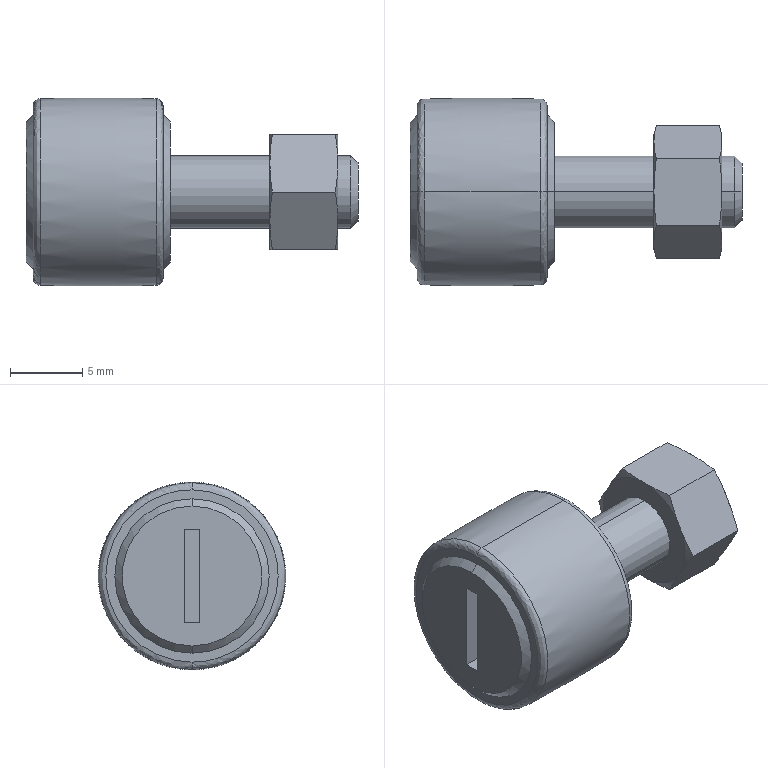Part | STEP file | CFU5-13 | 1 solid | 46 faces | box 23 x 13 x 13 mm | volume 1674 mm3 | plane 18 | cone 18 | spline 4 | cylinder 4 | torus 2 | commonest cylinder face diameters 5 x4
STEP:
#1=CARTESIAN_POINT('',(-0.992,0.,-6.468));
#2=VERTEX_POINT('',#1);
#3=CARTESIAN_POINT('',(-0.992,0.,6.468));
#4=VERTEX_POINT('',#3);
#5=CARTESIAN_POINT('',(-0.992,0.,0.));
#6=DIRECTION('',(-1.,0.,0.));
#7=DIRECTION('',(0.,0.,1.));
#8=AXIS2_PLACEMENT_3D('',#5,#6,#7);
#9=CIRCLE('',#8,6.468);
#10=EDGE_CURVE('',#2,#4,#9,.T.);
#11=ORIENTED_EDGE('',*,*,#10,.F.);
#12=CARTESIAN_POINT('',(-0.5,0.,-5.968));
#13=VERTEX_POINT('',#12);
#14=CARTESIAN_POINT('',(-1.,0.,-5.968));
#15=DIRECTION('',(0.,-1.,0.));
#16=DIRECTION('',(0.,0.,-1.));
#17=AXIS2_PLACEMENT_3D('',#14,#15,#16);
#18=CIRCLE('',#17,0.5);
#19=EDGE_CURVE('',#2,#13,#18,.T.);
#20=ORIENTED_EDGE('',*,*,#19,.T.);
#21=CARTESIAN_POINT('',(-0.5,0.,5.968));
#22=VERTEX_POINT('',#21);
#23=CARTESIAN_POINT('',(-0.5,0.,-5.968));
#24=CARTESIAN_POINT('',(-0.5,-11.936,-5.968));
#25=CARTESIAN_POINT('',(-0.5,-11.936,5.968));
#26=CARTESIAN_POINT('',(-0.5,0.,5.968));
#27=(BOUNDED_CURVE()B_SPLINE_CURVE(3,(#23,#24,#25,#26),.UNSPECIFIED.,.F.,.F.)B_SPLINE_CURVE_WITH_KNOTS((4,4),(0.,1.),.UNSPECIFIED.)CURVE()GEOMETRIC_REPRESENTATION_ITEM()RATIONAL_B_SPLINE_CURVE((1.,0.3333,0.3333,1.))REPRESENTATION_ITEM(''));
#28=EDGE_CURVE('',#13,#22,#27,.T.);
#29=ORIENTED_EDGE('',*,*,#28,.T.);
#30=CARTESIAN_POINT('',(-1.,0.,5.968));
#31=DIRECTION('',(0.,1.,0.));
#32=DIRECTION('',(0.,0.,1.));
#33=AXIS2_PLACEMENT_3D('',#30,#31,#32);
#34=CIRCLE('',#33,0.5);
#35=EDGE_CURVE('',#4,#22,#34,.T.);
#36=ORIENTED_EDGE('',*,*,#35,.F.);
#37=EDGE_LOOP('',(#11,#20,#29,#36));
#38=FACE_OUTER_BOUND('',#37,.T.);
#39=CARTESIAN_POINT('',(-0.992,0.,-6.468));
#40=CARTESIAN_POINT('',(-0.992,-12.936,-6.468));
#41=CARTESIAN_POINT('',(-0.992,-12.936,6.468));
#42=CARTESIAN_POINT('',(-0.992,0.,6.468));
#43=CARTESIAN_POINT('',(-0.7028,0.,-6.463));
#44=CARTESIAN_POINT('',(-0.7028,-12.926,-6.463));
#45=CARTESIAN_POINT('',(-0.7028,-12.926,6.463));
#46=CARTESIAN_POINT('',(-0.7028,0.,6.463));
#47=CARTESIAN_POINT('',(-0.5,0.,-6.257));
#48=CARTESIAN_POINT('',(-0.5,-12.514,-6.257));
#49=CARTESIAN_POINT('',(-0.5,-12.514,6.257));
#50=CARTESIAN_POINT('',(-0.5,0.,6.257));
#51=CARTESIAN_POINT('',(-0.5,0.,-5.968));
#52=CARTESIAN_POINT('',(-0.5,-11.936,-5.968));
#53=CARTESIAN_POINT('',(-0.5,-11.936,5.968));
#54=CARTESIAN_POINT('',(-0.5,0.,5.968));
#55=(BOUNDED_SURFACE()B_SPLINE_SURFACE(3,3,((#39,#40,#41,#42),(#43,#44,#45,#46),(#47,#48,#49,#50),(#51,#52,#53,#54)),.UNSPECIFIED.,.F.,.F.,.F.)B_SPLINE_SURFACE_WITH_KNOTS((4,4),(4,4),(0.,1.),(0.,1.),.UNSPECIFIED.)GEOMETRIC_REPRESENTATION_ITEM()RATIONAL_B_SPLINE_SURFACE(((1.,0.3333,0.3333,1.),(0.8085,0.2695,0.2695,0.8085),(0.8085,0.2695,0.2695,0.8085),(1.,0.3333,0.3333,1.)))REPRESENTATION_ITEM('')SURFACE());
#56=ADVANCED_FACE('',(#38),#55,.T.);
#57=CARTESIAN_POINT('',(-9.5,-5.968,0.));
#58=VERTEX_POINT('',#57);
#59=CARTESIAN_POINT('',(-9.5,0.,-5.968));
#60=VERTEX_POINT('',#59);
#61=CARTESIAN_POINT('',(-9.5,-5.968,0.));
#62=CARTESIAN_POINT('',(-9.5,-5.968,-3.496));
#63=CARTESIAN_POINT('',(-9.5,-3.496,-5.968));
#64=CARTESIAN_POINT('',(-9.5,0.,-5.968));
#65=(BOUNDED_CURVE()B_SPLINE_CURVE(3,(#61,#62,#63,#64),.UNSPECIFIED.,.F.,.F.)B_SPLINE_CURVE_WITH_KNOTS((4,4),(0.,1.),.UNSPECIFIED.)CURVE()GEOMETRIC_REPRESENTATION_ITEM()RATIONAL_B_SPLINE_CURVE((1.,0.8047,0.8047,1.))REPRESENTATION_ITEM(''));
#66=EDGE_CURVE('',#58,#60,#65,.T.);
#67=ORIENTED_EDGE('',*,*,#66,.T.);
#68=CARTESIAN_POINT('',(-9.008,0.,-6.468));
#69=VERTEX_POINT('',#68);
#70=CARTESIAN_POINT('',(-9.,0.,-5.968));
#71=DIRECTION('',(0.,-1.,0.));
#72=DIRECTION('',(0.,0.,-1.));
#73=AXIS2_PLACEMENT_3D('',#70,#71,#72);
#74=CIRCLE('',#73,0.5);
#75=EDGE_CURVE('',#60,#69,#74,.T.);
#76=ORIENTED_EDGE('',*,*,#75,.T.);
#77=CARTESIAN_POINT('',(-9.008,0.,6.468));
#78=VERTEX_POINT('',#77);
#79=CARTESIAN_POINT('',(-9.008,0.,0.));
#80=DIRECTION('',(1.,0.,0.));
#81=DIRECTION('',(0.,0.,-1.));
#82=AXIS2_PLACEMENT_3D('',#79,#80,#81);
#83=CIRCLE('',#82,6.468);
#84=EDGE_CURVE('',#78,#69,#83,.T.);
#85=ORIENTED_EDGE('',*,*,#84,.F.);
#86=CARTESIAN_POINT('',(-9.5,0.,5.968));
#87=VERTEX_POINT('',#86);
#88=CARTESIAN_POINT('',(-9.,0.,5.968));
#89=DIRECTION('',(0.,1.,0.));
#90=DIRECTION('',(0.,0.,1.));
#91=AXIS2_PLACEMENT_3D('',#88,#89,#90);
#92=CIRCLE('',#91,0.5);
#93=EDGE_CURVE('',#87,#78,#92,.T.);
#94=ORIENTED_EDGE('',*,*,#93,.F.);
#95=CARTESIAN_POINT('',(-9.5,0.,5.968));
#96=CARTESIAN_POINT('',(-9.5,-3.496,5.968));
#97=CARTESIAN_POINT('',(-9.5,-5.968,3.496));
#98=CARTESIAN_POINT('',(-9.5,-5.968,0.));
#99=(BOUNDED_CURVE()B_SPLINE_CURVE(3,(#95,#96,#97,#98),.UNSPECIFIED.,.F.,.F.)B_SPLINE_CURVE_WITH_KNOTS((4,4),(0.,1.),.UNSPECIFIED.)CURVE()GEOMETRIC_REPRESENTATION_ITEM()RATIONAL_B_SPLINE_CURVE((1.,0.8047,0.8047,1.))REPRESENTATION_ITEM(''));
#100=EDGE_CURVE('',#87,#58,#99,.T.);
#101=ORIENTED_EDGE('',*,*,#100,.T.);
#102=EDGE_LOOP('',(#67,#76,#85,#94,#101));
#103=FACE_OUTER_BOUND('',#102,.T.);
#104=CARTESIAN_POINT('',(-9.5,0.,-5.968));
#105=CARTESIAN_POINT('',(-9.5,-11.936,-5.968));
#106=CARTESIAN_POINT('',(-9.5,-11.936,5.968));
#107=CARTESIAN_POINT('',(-9.5,0.,5.968));
#108=CARTESIAN_POINT('',(-9.5,0.,-6.257));
#109=CARTESIAN_POINT('',(-9.5,-12.514,-6.257));
#110=CARTESIAN_POINT('',(-9.5,-12.514,6.257));
#111=CARTESIAN_POINT('',(-9.5,0.,6.257));
#112=CARTESIAN_POINT('',(-9.297,0.,-6.463));
#113=CARTESIAN_POINT('',(-9.297,-12.926,-6.463));
#114=CARTESIAN_POINT('',(-9.297,-12.926,6.463));
#115=CARTESIAN_POINT('',(-9.297,0.,6.463));
#116=CARTESIAN_POINT('',(-9.008,0.,-6.468));
#117=CARTESIAN_POINT('',(-9.008,-12.936,-6.468));
#118=CARTESIAN_POINT('',(-9.008,-12.936,6.468));
#119=CARTESIAN_POINT('',(-9.008,0.,6.468));
#120=(BOUNDED_SURFACE()B_SPLINE_SURFACE(3,3,((#104,#105,#106,#107),(#108,#109,#110,#111),(#112,#113,#114,#115),(#116,#117,#118,#119)),.UNSPECIFIED.,.F.,.F.,.F.)B_SPLINE_SURFACE_WITH_KNOTS((4,4),(4,4),(0.,1.),(0.,1.),.UNSPECIFIED.)GEOMETRIC_REPRESENTATION_ITEM()RATIONAL_B_SPLINE_SURFACE(((1.,0.3333,0.3333,1.),(0.8085,0.2695,0.2695,0.8085),(0.8085,0.2695,0.2695,0.8085),(1.,0.3333,0.3333,1.)))REPRESENTATION_ITEM('')SURFACE());
#121=ADVANCED_FACE('',(#103),#120,.T.);
#122=CARTESIAN_POINT('',(-0.992,0.,0.));
#123=DIRECTION('',(-1.,0.,0.));
#124=DIRECTION('',(0.,0.,1.));
#125=AXIS2_PLACEMENT_3D('',#122,#123,#124);
#126=CIRCLE('',#125,6.468);
#127=EDGE_CURVE('',#4,#2,#126,.T.);
#128=ORIENTED_EDGE('',*,*,#127,.T.);
#129=CARTESIAN_POINT('',(-5.,0.,243.5));
#130=DIRECTION('',(0.,1.,0.));
#131=DIRECTION('',(0.,0.,1.));
#132=AXIS2_PLACEMENT_3D('',#129,#130,#131);
#133=CIRCLE('',#132,250.);
#134=EDGE_CURVE('',#2,#69,#133,.T.);
#135=ORIENTED_EDGE('',*,*,#134,.T.);
#136=CARTESIAN_POINT('',(-9.008,0.,0.));
#137=DIRECTION('',(1.,0.,0.));
#138=DIRECTION('',(0.,0.,-1.));
#139=AXIS2_PLACEMENT_3D('',#136,#137,#138);
#140=CIRCLE('',#139,6.468);
#141=EDGE_CURVE('',#69,#78,#140,.T.);
#142=ORIENTED_EDGE('',*,*,#141,.T.);
#143=CARTESIAN_POINT('',(-5.,0.,-243.5));
#144=DIRECTION('',(0.,-1.,0.));
#145=DIRECTION('',(0.,0.,-1.));
#146=AXIS2_PLACEMENT_3D('',#143,#144,#145);
#147=CIRCLE('',#146,250.);
#148=EDGE_CURVE('',#4,#78,#147,.T.);
#149=ORIENTED_EDGE('',*,*,#148,.F.);
#150=EDGE_LOOP('',(#128,#135,#142,#149));
#151=FACE_OUTER_BOUND('',#150,.T.);
#152=CARTESIAN_POINT('',(-5.,0.,0.));
#153=DIRECTION('',(-1.,0.,0.));
#154=DIRECTION('',(0.,0.,1.));
#155=AXIS2_PLACEMENT_3D('',#152,#153,#154);
#156=TOROIDAL_SURFACE('',#155,-243.5,250.);
#157=ADVANCED_FACE('',(#151),#156,.T.);
#158=CARTESIAN_POINT('',(0.,0.,4.85));
#159=VERTEX_POINT('',#158);
#160=CARTESIAN_POINT('',(0.,0.,-4.85));
#161=VERTEX_POINT('',#160);
#162=CARTESIAN_POINT('',(0.,0.,0.));
#163=DIRECTION('',(-1.,0.,0.));
#164=DIRECTION('',(0.,0.,1.));
#165=AXIS2_PLACEMENT_3D('',#162,#163,#164);
#166=CIRCLE('',#165,4.85);
#167=EDGE_CURVE('',#159,#161,#166,.T.);
#168=ORIENTED_EDGE('',*,*,#167,.T.);
#169=CARTESIAN_POINT('',(-0.5,0.,-5.35));
#170=VERTEX_POINT('',#169);
#171=CARTESIAN_POINT('',(-0.5,0.,-5.35));
#172=DIRECTION('',(-0.7071,0.,-0.7071));
#173=VECTOR('',#172,1000.);
#174=LINE('',#171,#173);
#175=EDGE_CURVE('',#161,#170,#174,.T.);
#176=ORIENTED_EDGE('',*,*,#175,.T.);
#177=CARTESIAN_POINT('',(-0.5,0.,5.35));
#178=VERTEX_POINT('',#177);
#179=CARTESIAN_POINT('',(-0.5,0.,0.));
#180=DIRECTION('',(-1.,0.,0.));
#181=DIRECTION('',(0.,0.,1.));
#182=AXIS2_PLACEMENT_3D('',#179,#180,#181);
#183=CIRCLE('',#182,5.35);
#184=EDGE_CURVE('',#178,#170,#183,.T.);
#185=ORIENTED_EDGE('',*,*,#184,.F.);
#186=CARTESIAN_POINT('',(-0.5,0.,5.35));
#187=DIRECTION('',(-0.7071,0.,0.7071));
#188=VECTOR('',#187,1000.);
#189=LINE('',#186,#188);
#190=EDGE_CURVE('',#159,#178,#189,.T.);
#191=ORIENTED_EDGE('',*,*,#190,.F.);
#192=EDGE_LOOP('',(#168,#176,#185,#191));
#193=FACE_OUTER_BOUND('',#192,.T.);
#194=CARTESIAN_POINT('',(-0.5,0.,0.));
#195=DIRECTION('',(-1.,0.,0.));
#196=DIRECTION('',(0.,0.,1.));
#197=AXIS2_PLACEMENT_3D('',#194,#195,#196);
#198=CONICAL_SURFACE('',#197,5.35,0.7854);
#199=ADVANCED_FACE('',(#193),#198,.T.);
#200=CARTESIAN_POINT('',(-10.,0.,-4.85));
#201=VERTEX_POINT('',#200);
#202=CARTESIAN_POINT('',(-10.,0.,4.85));
#203=VERTEX_POINT('',#202);
#204=CARTESIAN_POINT('',(-10.,0.,0.));
#205=DIRECTION('',(1.,0.,0.));
#206=DIRECTION('',(0.,0.,-1.));
#207=AXIS2_PLACEMENT_3D('',#204,#205,#206);
#208=CIRCLE('',#207,4.85);
#209=EDGE_CURVE('',#201,#203,#208,.T.);
#210=ORIENTED_EDGE('',*,*,#209,.T.);
#211=CARTESIAN_POINT('',(-9.5,0.,5.35));
#212=VERTEX_POINT('',#211);
#213=CARTESIAN_POINT('',(-9.5,0.,5.35));
#214=DIRECTION('',(0.7071,0.,0.7071));
#215=VECTOR('',#214,1000.);
#216=LINE('',#213,#215);
#217=EDGE_CURVE('',#203,#212,#216,.T.);
#218=ORIENTED_EDGE('',*,*,#217,.T.);
#219=CARTESIAN_POINT('',(-9.5,0.,-5.35));
#220=VERTEX_POINT('',#219);
#221=CARTESIAN_POINT('',(-9.5,0.,0.));
#222=DIRECTION('',(1.,0.,0.));
#223=DIRECTION('',(0.,0.,-1.));
#224=AXIS2_PLACEMENT_3D('',#221,#222,#223);
#225=CIRCLE('',#224,5.35);
#226=EDGE_CURVE('',#220,#212,#225,.T.);
#227=ORIENTED_EDGE('',*,*,#226,.F.);
#228=CARTESIAN_POINT('',(-9.5,0.,-5.35));
#229=DIRECTION('',(0.7071,0.,-0.7071));
#230=VECTOR('',#229,1000.);
#231=LINE('',#228,#230);
#232=EDGE_CURVE('',#201,#220,#231,.T.);
#233=ORIENTED_EDGE('',*,*,#232,.F.);
#234=EDGE_LOOP('',(#210,#218,#227,#233));
#235=FACE_OUTER_BOUND('',#234,.T.);
#236=CARTESIAN_POINT('',(-9.5,0.,0.));
#237=DIRECTION('',(1.,0.,0.));
#238=DIRECTION('',(0.,0.,-1.));
#239=AXIS2_PLACEMENT_3D('',#236,#237,#238);
#240=CONICAL_SURFACE('',#239,5.35,0.7854);
#241=ADVANCED_FACE('',(#235),#240,.T.);
#242=CARTESIAN_POINT('',(0.,0.,2.5));
#243=VERTEX_POINT('',#242);
#244=CARTESIAN_POINT('',(0.,0.,-2.5));
#245=VERTEX_POINT('',#244);
#246=CARTESIAN_POINT('',(0.,0.,0.));
#247=DIRECTION('',(-1.,0.,0.));
#248=DIRECTION('',(0.,0.,-1.));
#249=AXIS2_PLACEMENT_3D('',#246,#247,#248);
#250=CIRCLE('',#249,2.5);
#251=EDGE_CURVE('',#243,#245,#250,.T.);
#252=ORIENTED_EDGE('',*,*,#251,.F.);
#253=CARTESIAN_POINT('',(6.9,0.,2.5));
#254=VERTEX_POINT('',#253);
#255=CARTESIAN_POINT('',(6.255,0.,2.5));
#256=DIRECTION('',(1.,0.,0.));
#257=VECTOR('',#256,1000.);
#258=LINE('',#255,#257);
#259=EDGE_CURVE('',#243,#254,#258,.T.);
#260=ORIENTED_EDGE('',*,*,#259,.T.);
#261=CARTESIAN_POINT('',(6.9,0.,-2.5));
#262=VERTEX_POINT('',#261);
#263=CARTESIAN_POINT('',(6.9,0.,0.));
#264=DIRECTION('',(-1.,0.,0.));
#265=DIRECTION('',(0.,0.,-1.));
#266=AXIS2_PLACEMENT_3D('',#263,#264,#265);
#267=CIRCLE('',#266,2.5);
#268=EDGE_CURVE('',#254,#262,#267,.T.);
#269=ORIENTED_EDGE('',*,*,#268,.T.);
#270=CARTESIAN_POINT('',(6.255,0.,-2.5));
#271=DIRECTION('',(1.,0.,0.));
#272=VECTOR('',#271,1000.);
#273=LINE('',#270,#272);
#274=EDGE_CURVE('',#245,#262,#273,.T.);
#275=ORIENTED_EDGE('',*,*,#274,.F.);
#276=EDGE_LOOP('',(#252,#260,#269,#275));
#277=FACE_OUTER_BOUND('',#276,.T.);
#278=CARTESIAN_POINT('',(6.255,0.,0.));
#279=DIRECTION('',(1.,0.,0.));
#280=DIRECTION('',(0.,0.,-1.));
#281=AXIS2_PLACEMENT_3D('',#278,#279,#280);
#282=CYLINDRICAL_SURFACE('',#281,2.5);
#283=ADVANCED_FACE('',(#277),#282,.T.);
#284=CARTESIAN_POINT('',(11.6,0.,-2.5));
#285=VERTEX_POINT('',#284);
#286=CARTESIAN_POINT('',(11.6,0.,2.5));
#287=VERTEX_POINT('',#286);
#288=CARTESIAN_POINT('',(11.6,0.,0.));
#289=DIRECTION('',(1.,0.,0.));
#290=DIRECTION('',(0.,0.,-1.));
#291=AXIS2_PLACEMENT_3D('',#288,#289,#290);
#292=CIRCLE('',#291,2.5);
#293=EDGE_CURVE('',#285,#287,#292,.T.);
#294=ORIENTED_EDGE('',*,*,#293,.T.);
#295=CARTESIAN_POINT('',(12.509,0.,2.5));
#296=VERTEX_POINT('',#295);
#297=CARTESIAN_POINT('',(6.255,0.,2.5));
#298=DIRECTION('',(1.,0.,0.));
#299=VECTOR('',#298,1000.);
#300=LINE('',#297,#299);
#301=EDGE_CURVE('',#287,#296,#300,.T.);
#302=ORIENTED_EDGE('',*,*,#301,.T.);
#303=CARTESIAN_POINT('',(12.509,0.,-2.5));
#304=VERTEX_POINT('',#303);
#305=CARTESIAN_POINT('',(12.509,0.,0.));
#306=DIRECTION('',(-1.,0.,0.));
#307=DIRECTION('',(0.,0.,-1.));
#308=AXIS2_PLACEMENT_3D('',#305,#306,#307);
#309=CIRCLE('',#308,2.5);
#310=EDGE_CURVE('',#296,#304,#309,.T.);
#311=ORIENTED_EDGE('',*,*,#310,.T.);
#312=CARTESIAN_POINT('',(6.255,0.,-2.5));
#313=DIRECTION('',(1.,0.,0.));
#314=VECTOR('',#313,1000.);
#315=LINE('',#312,#314);
#316=EDGE_CURVE('',#285,#304,#315,.T.);
#317=ORIENTED_EDGE('',*,*,#316,.F.);
#318=EDGE_LOOP('',(#294,#302,#311,#317));
#319=FACE_OUTER_BOUND('',#318,.T.);
#320=CARTESIAN_POINT('',(6.255,0.,0.));
#321=DIRECTION('',(1.,0.,0.));
#322=DIRECTION('',(0.,0.,-1.));
#323=AXIS2_PLACEMENT_3D('',#320,#321,#322);
#324=CYLINDRICAL_SURFACE('',#323,2.5);
#325=ADVANCED_FACE('',(#319),#324,.T.);
#326=CARTESIAN_POINT('',(13.,0.,2.009));
#327=VERTEX_POINT('',#326);
#328=CARTESIAN_POINT('',(13.,0.,-2.009));
#329=VERTEX_POINT('',#328);
#330=CARTESIAN_POINT('',(13.,0.,0.));
#331=DIRECTION('',(-1.,0.,0.));
#332=DIRECTION('',(0.,0.,1.));
#333=AXIS2_PLACEMENT_3D('',#330,#331,#332);
#334=CIRCLE('',#333,2.009);
#335=EDGE_CURVE('',#327,#329,#334,.T.);
#336=ORIENTED_EDGE('',*,*,#335,.T.);
#337=CARTESIAN_POINT('',(12.51,0.,-2.5));
#338=DIRECTION('',(-0.7071,0.,-0.7071));
#339=VECTOR('',#338,1000.);
#340=LINE('',#337,#339);
#341=EDGE_CURVE('',#329,#304,#340,.T.);
#342=ORIENTED_EDGE('',*,*,#341,.T.);
#343=ORIENTED_EDGE('',*,*,#310,.F.);
#344=CARTESIAN_POINT('',(12.51,0.,2.5));
#345=DIRECTION('',(-0.7071,0.,0.7071));
#346=VECTOR('',#345,1000.);
#347=LINE('',#344,#346);
#348=EDGE_CURVE('',#327,#296,#347,.T.);
#349=ORIENTED_EDGE('',*,*,#348,.F.);
#350=EDGE_LOOP('',(#336,#342,#343,#349));
#351=FACE_OUTER_BOUND('',#350,.T.);
#352=CARTESIAN_POINT('',(12.51,0.,0.));
#353=DIRECTION('',(-1.,0.,0.));
#354=DIRECTION('',(0.,0.,1.));
#355=AXIS2_PLACEMENT_3D('',#352,#353,#354);
#356=CONICAL_SURFACE('',#355,2.5,0.7854);
#357=ADVANCED_FACE('',(#351),#356,.T.);
#358=ORIENTED_EDGE('',*,*,#134,.F.);
#359=ORIENTED_EDGE('',*,*,#10,.T.);
#360=ORIENTED_EDGE('',*,*,#148,.T.);
#361=ORIENTED_EDGE('',*,*,#84,.T.);
#362=EDGE_LOOP('',(#358,#359,#360,#361));
#363=FACE_OUTER_BOUND('',#362,.T.);
#364=CARTESIAN_POINT('',(-5.,0.,0.));
#365=DIRECTION('',(-1.,0.,0.));
#366=DIRECTION('',(0.,0.,1.));
#367=AXIS2_PLACEMENT_3D('',#364,#365,#366);
#368=TOROIDAL_SURFACE('',#367,-243.5,250.);
#369=ADVANCED_FACE('',(#363),#368,.T.);
#370=ORIENTED_EDGE('',*,*,#19,.F.);
#371=ORIENTED_EDGE('',*,*,#127,.F.);
#372=ORIENTED_EDGE('',*,*,#35,.T.);
#373=CARTESIAN_POINT('',(-0.5,5.968,0.));
#374=VERTEX_POINT('',#373);
#375=CARTESIAN_POINT('',(-0.5,0.,5.968));
#376=CARTESIAN_POINT('',(-0.5,3.496,5.968));
#377=CARTESIAN_POINT('',(-0.5,5.968,3.496));
#378=CARTESIAN_POINT('',(-0.5,5.968,0.));
#379=(BOUNDED_CURVE()B_SPLINE_CURVE(3,(#375,#376,#377,#378),.UNSPECIFIED.,.F.,.F.)B_SPLINE_CURVE_WITH_KNOTS((4,4),(0.,1.),.UNSPECIFIED.)CURVE()GEOMETRIC_REPRESENTATION_ITEM()RATIONAL_B_SPLINE_CURVE((1.,0.8047,0.8047,1.))REPRESENTATION_ITEM(''));
#380=EDGE_CURVE('',#22,#374,#379,.T.);
#381=ORIENTED_EDGE('',*,*,#380,.T.);
#382=CARTESIAN_POINT('',(-0.5,5.968,0.));
#383=CARTESIAN_POINT('',(-0.5,5.968,-3.496));
#384=CARTESIAN_POINT('',(-0.5,3.496,-5.968));
#385=CARTESIAN_POINT('',(-0.5,0.,-5.968));
#386=(BOUNDED_CURVE()B_SPLINE_CURVE(3,(#382,#383,#384,#385),.UNSPECIFIED.,.F.,.F.)B_SPLINE_CURVE_WITH_KNOTS((4,4),(0.,1.),.UNSPECIFIED.)CURVE()GEOMETRIC_REPRESENTATION_ITEM()RATIONAL_B_SPLINE_CURVE((1.,0.8047,0.8047,1.))REPRESENTATION_ITEM(''));
#387=EDGE_CURVE('',#374,#13,#386,.T.);
#388=ORIENTED_EDGE('',*,*,#387,.T.);
#389=EDGE_LOOP('',(#370,#371,#372,#381,#388));
#390=FACE_OUTER_BOUND('',#389,.T.);
#391=CARTESIAN_POINT('',(-0.992,0.,6.468));
#392=CARTESIAN_POINT('',(-0.992,12.936,6.468));
#393=CARTESIAN_POINT('',(-0.992,12.936,-6.468));
#394=CARTESIAN_POINT('',(-0.992,0.,-6.468));
#395=CARTESIAN_POINT('',(-0.7028,0.,6.463));
#396=CARTESIAN_POINT('',(-0.7028,12.926,6.463));
#397=CARTESIAN_POINT('',(-0.7028,12.926,-6.463));
#398=CARTESIAN_POINT('',(-0.7028,0.,-6.463));
#399=CARTESIAN_POINT('',(-0.5,0.,6.257));
#400=CARTESIAN_POINT('',(-0.5,12.514,6.257));
#401=CARTESIAN_POINT('',(-0.5,12.514,-6.257));
#402=CARTESIAN_POINT('',(-0.5,0.,-6.257));
#403=CARTESIAN_POINT('',(-0.5,0.,5.968));
#404=CARTESIAN_POINT('',(-0.5,11.936,5.968));
#405=CARTESIAN_POINT('',(-0.5,11.936,-5.968));
#406=CARTESIAN_POINT('',(-0.5,0.,-5.968));
#407=(BOUNDED_SURFACE()B_SPLINE_SURFACE(3,3,((#391,#392,#393,#394),(#395,#396,#397,#398),(#399,#400,#401,#402),(#403,#404,#405,#406)),.UNSPECIFIED.,.F.,.F.,.F.)B_SPLINE_SURFACE_WITH_KNOTS((4,4),(4,4),(0.,1.),(0.,1.),.UNSPECIFIED.)GEOMETRIC_REPRESENTATION_ITEM()RATIONAL_B_SPLINE_SURFACE(((1.,0.3333,0.3333,1.),(0.8085,0.2695,0.2695,0.8085),(0.8085,0.2695,0.2695,0.8085),(1.,0.3333,0.3333,1.)))REPRESENTATION_ITEM('')SURFACE());
#408=ADVANCED_FACE('',(#390),#407,.T.);
#409=ORIENTED_EDGE('',*,*,#75,.F.);
#410=CARTESIAN_POINT('',(-9.5,5.968,0.));
#411=VERTEX_POINT('',#410);
#412=CARTESIAN_POINT('',(-9.5,0.,-5.968));
#413=CARTESIAN_POINT('',(-9.5,3.496,-5.968));
#414=CARTESIAN_POINT('',(-9.5,5.968,-3.496));
#415=CARTESIAN_POINT('',(-9.5,5.968,0.));
#416=(BOUNDED_CURVE()B_SPLINE_CURVE(3,(#412,#413,#414,#415),.UNSPECIFIED.,.F.,.F.)B_SPLINE_CURVE_WITH_KNOTS((4,4),(0.,1.),.UNSPECIFIED.)CURVE()GEOMETRIC_REPRESENTATION_ITEM()RATIONAL_B_SPLINE_CURVE((1.,0.8047,0.8047,1.))REPRESENTATION_ITEM(''));
#417=EDGE_CURVE('',#60,#411,#416,.T.);
#418=ORIENTED_EDGE('',*,*,#417,.T.);
#419=CARTESIAN_POINT('',(-9.5,5.968,0.));
#420=CARTESIAN_POINT('',(-9.5,5.968,3.496));
#421=CARTESIAN_POINT('',(-9.5,3.496,5.968));
#422=CARTESIAN_POINT('',(-9.5,0.,5.968));
#423=(BOUNDED_CURVE()B_SPLINE_CURVE(3,(#419,#420,#421,#422),.UNSPECIFIED.,.F.,.T.)B_SPLINE_CURVE_WITH_KNOTS((4,4),(0.,1.),.UNSPECIFIED.)CURVE()GEOMETRIC_REPRESENTATION_ITEM()RATIONAL_B_SPLINE_CURVE((1.,0.8047,0.8047,1.))REPRESENTATION_ITEM(''));
#424=EDGE_CURVE('',#411,#87,#423,.T.);
#425=ORIENTED_EDGE('',*,*,#424,.T.);
#426=ORIENTED_EDGE('',*,*,#93,.T.);
#427=ORIENTED_EDGE('',*,*,#141,.F.);
#428=EDGE_LOOP('',(#409,#418,#425,#426,#427));
#429=FACE_OUTER_BOUND('',#428,.T.);
#430=CARTESIAN_POINT('',(-9.5,0.,5.968));
#431=CARTESIAN_POINT('',(-9.5,11.936,5.968));
#432=CARTESIAN_POINT('',(-9.5,11.936,-5.968));
#433=CARTESIAN_POINT('',(-9.5,0.,-5.968));
#434=CARTESIAN_POINT('',(-9.5,0.,6.257));
#435=CARTESIAN_POINT('',(-9.5,12.514,6.257));
#436=CARTESIAN_POINT('',(-9.5,12.514,-6.257));
#437=CARTESIAN_POINT('',(-9.5,0.,-6.257));
#438=CARTESIAN_POINT('',(-9.297,0.,6.463));
#439=CARTESIAN_POINT('',(-9.297,12.926,6.463));
#440=CARTESIAN_POINT('',(-9.297,12.926,-6.463));
#441=CARTESIAN_POINT('',(-9.297,0.,-6.463));
#442=CARTESIAN_POINT('',(-9.008,0.,6.468));
#443=CARTESIAN_POINT('',(-9.008,12.936,6.468));
#444=CARTESIAN_POINT('',(-9.008,12.936,-6.468));
#445=CARTESIAN_POINT('',(-9.008,0.,-6.468));
#446=(BOUNDED_SURFACE()B_SPLINE_SURFACE(3,3,((#430,#431,#432,#433),(#434,#435,#436,#437),(#438,#439,#440,#441),(#442,#443,#444,#445)),.UNSPECIFIED.,.F.,.F.,.F.)B_SPLINE_SURFACE_WITH_KNOTS((4,4),(4,4),(0.,1.),(0.,1.),.UNSPECIFIED.)GEOMETRIC_REPRESENTATION_ITEM()RATIONAL_B_SPLINE_SURFACE(((1.,0.3333,0.3333,1.),(0.8085,0.2695,0.2695,0.8085),(0.8085,0.2695,0.2695,0.8085),(1.,0.3333,0.3333,1.)))REPRESENTATION_ITEM('')SURFACE());
#447=ADVANCED_FACE('',(#429),#446,.T.);
#448=ORIENTED_EDGE('',*,*,#184,.T.);
#449=CARTESIAN_POINT('',(-0.5,0.,0.));
#450=DIRECTION('',(-1.,0.,0.));
#451=DIRECTION('',(0.,0.,1.));
#452=AXIS2_PLACEMENT_3D('',#449,#450,#451);
#453=CIRCLE('',#452,5.35);
#454=EDGE_CURVE('',#170,#178,#453,.T.);
#455=ORIENTED_EDGE('',*,*,#454,.T.);
#456=EDGE_LOOP('',(#448,#455));
#457=FACE_BOUND('',#456,.T.);
#458=ORIENTED_EDGE('',*,*,#28,.F.);
#459=ORIENTED_EDGE('',*,*,#387,.F.);
#460=ORIENTED_EDGE('',*,*,#380,.F.);
#461=EDGE_LOOP('',(#458,#459,#460));
#462=FACE_OUTER_BOUND('',#461,.T.);
#463=CARTESIAN_POINT('',(-0.5,5.659,0.));
#464=DIRECTION('',(1.,0.,0.));
#465=DIRECTION('',(0.,0.,-1.));
#466=AXIS2_PLACEMENT_3D('',#463,#464,#465);
#467=PLANE('',#466);
#468=ADVANCED_FACE('',(#457,#462),#467,.T.);
#469=ORIENTED_EDGE('',*,*,#226,.T.);
#470=CARTESIAN_POINT('',(-9.5,0.,0.));
#471=DIRECTION('',(1.,0.,0.));
#472=DIRECTION('',(0.,0.,-1.));
#473=AXIS2_PLACEMENT_3D('',#470,#471,#472);
#474=CIRCLE('',#473,5.35);
#475=EDGE_CURVE('',#212,#220,#474,.T.);
#476=ORIENTED_EDGE('',*,*,#475,.T.);
#477=EDGE_LOOP('',(#469,#476));
#478=FACE_BOUND('',#477,.T.);
#479=ORIENTED_EDGE('',*,*,#424,.F.);
#480=ORIENTED_EDGE('',*,*,#417,.F.);
#481=ORIENTED_EDGE('',*,*,#66,.F.);
#482=ORIENTED_EDGE('',*,*,#100,.F.);
#483=EDGE_LOOP('',(#479,#480,#481,#482));
#484=FACE_OUTER_BOUND('',#483,.T.);
#485=CARTESIAN_POINT('',(-9.5,5.659,0.));
#486=DIRECTION('',(-1.,0.,0.));
#487=DIRECTION('',(0.,0.,1.));
#488=AXIS2_PLACEMENT_3D('',#485,#486,#487);
#489=PLANE('',#488);
#490=ADVANCED_FACE('',(#478,#484),#489,.T.);
#491=ORIENTED_EDGE('',*,*,#175,.F.);
#492=CARTESIAN_POINT('',(0.,0.,0.));
#493=DIRECTION('',(-1.,0.,0.));
#494=DIRECTION('',(0.,0.,1.));
#495=AXIS2_PLACEMENT_3D('',#492,#493,#494);
#496=CIRCLE('',#495,4.85);
#497=EDGE_CURVE('',#161,#159,#496,.T.);
#498=ORIENTED_EDGE('',*,*,#497,.T.);
#499=ORIENTED_EDGE('',*,*,#190,.T.);
#500=ORIENTED_EDGE('',*,*,#454,.F.);
#501=EDGE_LOOP('',(#491,#498,#499,#500));
#502=FACE_OUTER_BOUND('',#501,.T.);
#503=CARTESIAN_POINT('',(-0.5,0.,0.));
#504=DIRECTION('',(-1.,0.,0.));
#505=DIRECTION('',(0.,0.,1.));
#506=AXIS2_PLACEMENT_3D('',#503,#504,#505);
#507=CONICAL_SURFACE('',#506,5.35,0.7854);
#508=ADVANCED_FACE('',(#502),#507,.T.);
#509=ORIENTED_EDGE('',*,*,#217,.F.);
#510=CARTESIAN_POINT('',(-10.,0.,0.));
#511=DIRECTION('',(1.,0.,0.));
#512=DIRECTION('',(0.,0.,-1.));
#513=AXIS2_PLACEMENT_3D('',#510,#511,#512);
#514=CIRCLE('',#513,4.85);
#515=EDGE_CURVE('',#203,#201,#514,.T.);
#516=ORIENTED_EDGE('',*,*,#515,.T.);
#517=ORIENTED_EDGE('',*,*,#232,.T.);
#518=ORIENTED_EDGE('',*,*,#475,.F.);
#519=EDGE_LOOP('',(#509,#516,#517,#518));
#520=FACE_OUTER_BOUND('',#519,.T.);
#521=CARTESIAN_POINT('',(-9.5,0.,0.));
#522=DIRECTION('',(1.,0.,0.));
#523=DIRECTION('',(0.,0.,-1.));
#524=AXIS2_PLACEMENT_3D('',#521,#522,#523);
#525=CONICAL_SURFACE('',#524,5.35,0.7854);
#526=ADVANCED_FACE('',(#520),#525,.T.);
#527=CARTESIAN_POINT('',(0.,0.,0.));
#528=DIRECTION('',(-1.,0.,0.));
#529=DIRECTION('',(0.,0.,-1.));
#530=AXIS2_PLACEMENT_3D('',#527,#528,#529);
#531=CIRCLE('',#530,2.5);
#532=EDGE_CURVE('',#245,#243,#531,.T.);
#533=ORIENTED_EDGE('',*,*,#532,.T.);
#534=ORIENTED_EDGE('',*,*,#251,.T.);
#535=EDGE_LOOP('',(#533,#534));
#536=FACE_BOUND('',#535,.T.);
#537=ORIENTED_EDGE('',*,*,#167,.F.);
#538=ORIENTED_EDGE('',*,*,#497,.F.);
#539=EDGE_LOOP('',(#537,#538));
#540=FACE_OUTER_BOUND('',#539,.T.);
#541=CARTESIAN_POINT('',(0.,3.675,0.));
#542=DIRECTION('',(1.,0.,0.));
#543=DIRECTION('',(0.,0.,-1.));
#544=AXIS2_PLACEMENT_3D('',#541,#542,#543);
#545=PLANE('',#544);
#546=ADVANCED_FACE('',(#536,#540),#545,.T.);
#547=CARTESIAN_POINT('',(-10.,-0.5417,-3.25));
#548=VERTEX_POINT('',#547);
#549=CARTESIAN_POINT('',(-10.,0.5417,-3.25));
#550=VERTEX_POINT('',#549);
#551=CARTESIAN_POINT('',(-10.,0.5417,-3.25));
#552=DIRECTION('',(0.,1.,0.));
#553=VECTOR('',#552,1000.);
#554=LINE('',#551,#553);
#555=EDGE_CURVE('',#548,#550,#554,.T.);
#556=ORIENTED_EDGE('',*,*,#555,.T.);
#557=CARTESIAN_POINT('',(-10.,0.5417,3.25));
#558=VERTEX_POINT('',#557);
#559=CARTESIAN_POINT('',(-10.,0.5417,0.));
#560=DIRECTION('',(0.,0.,1.));
#561=VECTOR('',#560,1000.);
#562=LINE('',#559,#561);
#563=EDGE_CURVE('',#550,#558,#562,.T.);
#564=ORIENTED_EDGE('',*,*,#563,.T.);
#565=CARTESIAN_POINT('',(-10.,-0.5417,3.25));
#566=VERTEX_POINT('',#565);
#567=CARTESIAN_POINT('',(-10.,-0.5417,3.25));
#568=DIRECTION('',(0.,-1.,0.));
#569=VECTOR('',#568,1000.);
#570=LINE('',#567,#569);
#571=EDGE_CURVE('',#558,#566,#570,.T.);
#572=ORIENTED_EDGE('',*,*,#571,.T.);
#573=CARTESIAN_POINT('',(-10.,-0.5417,0.));
#574=DIRECTION('',(0.,0.,-1.));
#575=VECTOR('',#574,1000.);
#576=LINE('',#573,#575);
#577=EDGE_CURVE('',#566,#548,#576,.T.);
#578=ORIENTED_EDGE('',*,*,#577,.T.);
#579=EDGE_LOOP('',(#556,#564,#572,#578));
#580=FACE_BOUND('',#579,.T.);
#581=ORIENTED_EDGE('',*,*,#209,.F.);
#582=ORIENTED_EDGE('',*,*,#515,.F.);
#583=EDGE_LOOP('',(#581,#582));
#584=FACE_OUTER_BOUND('',#583,.T.);
#585=CARTESIAN_POINT('',(-10.,2.425,0.));
#586=DIRECTION('',(-1.,0.,0.));
#587=DIRECTION('',(0.,0.,1.));
#588=AXIS2_PLACEMENT_3D('',#585,#586,#587);
#589=PLANE('',#588);
#590=ADVANCED_FACE('',(#580,#584),#589,.T.);
#591=ORIENTED_EDGE('',*,*,#259,.F.);
#592=ORIENTED_EDGE('',*,*,#532,.F.);
#593=ORIENTED_EDGE('',*,*,#274,.T.);
#594=CARTESIAN_POINT('',(6.9,0.,0.));
#595=DIRECTION('',(-1.,0.,0.));
#596=DIRECTION('',(0.,0.,-1.));
#597=AXIS2_PLACEMENT_3D('',#594,#595,#596);
#598=CIRCLE('',#597,2.5);
#599=EDGE_CURVE('',#262,#254,#598,.T.);
#600=ORIENTED_EDGE('',*,*,#599,.T.);
#601=EDGE_LOOP('',(#591,#592,#593,#600));
#602=FACE_OUTER_BOUND('',#601,.T.);
#603=CARTESIAN_POINT('',(6.255,0.,0.));
#604=DIRECTION('',(1.,0.,0.));
#605=DIRECTION('',(0.,0.,-1.));
#606=AXIS2_PLACEMENT_3D('',#603,#604,#605);
#607=CYLINDRICAL_SURFACE('',#606,2.5);
#608=ADVANCED_FACE('',(#602),#607,.T.);
#609=ORIENTED_EDGE('',*,*,#563,.F.);
#610=CARTESIAN_POINT('',(-8.,0.5417,-3.25));
#611=VERTEX_POINT('',#610);
#612=CARTESIAN_POINT('',(-10.,0.5417,-3.25));
#613=DIRECTION('',(-1.,0.,0.));
#614=VECTOR('',#613,1000.);
#615=LINE('',#612,#614);
#616=EDGE_CURVE('',#611,#550,#615,.T.);
#617=ORIENTED_EDGE('',*,*,#616,.F.);
#618=CARTESIAN_POINT('',(-8.,0.5417,3.25));
#619=VERTEX_POINT('',#618);
#620=CARTESIAN_POINT('',(-8.,0.5417,3.25));
#621=DIRECTION('',(0.,0.,-1.));
#622=VECTOR('',#621,1000.);
#623=LINE('',#620,#622);
#624=EDGE_CURVE('',#619,#611,#623,.T.);
#625=ORIENTED_EDGE('',*,*,#624,.F.);
#626=CARTESIAN_POINT('',(-10.,0.5417,3.25));
#627=DIRECTION('',(1.,0.,0.));
#628=VECTOR('',#627,1000.);
#629=LINE('',#626,#628);
#630=EDGE_CURVE('',#558,#619,#629,.T.);
#631=ORIENTED_EDGE('',*,*,#630,.F.);
#632=EDGE_LOOP('',(#609,#617,#625,#631));
#633=FACE_OUTER_BOUND('',#632,.T.);
#634=CARTESIAN_POINT('',(-10.,0.5417,3.25));
#635=DIRECTION('',(0.,1.,0.));
#636=DIRECTION('',(0.,0.,1.));
#637=AXIS2_PLACEMENT_3D('',#634,#635,#636);
#638=PLANE('',#637);
#639=ADVANCED_FACE('',(#633),#638,.F.);
#640=ORIENTED_EDGE('',*,*,#577,.F.);
#641=CARTESIAN_POINT('',(-8.,-0.5417,3.25));
#642=VERTEX_POINT('',#641);
#643=CARTESIAN_POINT('',(-10.,-0.5417,3.25));
#644=DIRECTION('',(-1.,0.,0.));
#645=VECTOR('',#644,1000.);
#646=LINE('',#643,#645);
#647=EDGE_CURVE('',#642,#566,#646,.T.);
#648=ORIENTED_EDGE('',*,*,#647,.F.);
#649=CARTESIAN_POINT('',(-8.,-0.5417,-3.25));
#650=VERTEX_POINT('',#649);
#651=CARTESIAN_POINT('',(-8.,-0.5417,-3.25));
#652=DIRECTION('',(0.,0.,1.));
#653=VECTOR('',#652,1000.);
#654=LINE('',#651,#653);
#655=EDGE_CURVE('',#650,#642,#654,.T.);
#656=ORIENTED_EDGE('',*,*,#655,.F.);
#657=CARTESIAN_POINT('',(-10.,-0.5417,-3.25));
#658=DIRECTION('',(1.,0.,0.));
#659=VECTOR('',#658,1000.);
#660=LINE('',#657,#659);
#661=EDGE_CURVE('',#548,#650,#660,.T.);
#662=ORIENTED_EDGE('',*,*,#661,.F.);
#663=EDGE_LOOP('',(#640,#648,#656,#662));
#664=FACE_OUTER_BOUND('',#663,.T.);
#665=CARTESIAN_POINT('',(-10.,-0.5417,-3.25));
#666=DIRECTION('',(0.,-1.,0.));
#667=DIRECTION('',(0.,0.,-1.));
#668=AXIS2_PLACEMENT_3D('',#665,#666,#667);
#669=PLANE('',#668);
#670=ADVANCED_FACE('',(#664),#669,.F.);
#671=ORIENTED_EDGE('',*,*,#599,.F.);
#672=ORIENTED_EDGE('',*,*,#268,.F.);
#673=EDGE_LOOP('',(#671,#672));
#674=FACE_BOUND('',#673,.T.);
#675=CARTESIAN_POINT('',(6.9,-3.464,-2.));
#676=VERTEX_POINT('',#675);
#677=CARTESIAN_POINT('',(6.9,-3.464,2.));
#678=VERTEX_POINT('',#677);
#679=CARTESIAN_POINT('',(6.9,0.,0.));
#680=DIRECTION('',(-1.,0.,0.));
#681=DIRECTION('',(0.,0.,-1.));
#682=AXIS2_PLACEMENT_3D('',#679,#680,#681);
#683=CIRCLE('',#682,4.);
#684=EDGE_CURVE('',#676,#678,#683,.T.);
#685=ORIENTED_EDGE('',*,*,#684,.T.);
#686=CARTESIAN_POINT('',(6.9,0.,4.));
#687=VERTEX_POINT('',#686);
#688=CARTESIAN_POINT('',(6.9,0.,0.));
#689=DIRECTION('',(-1.,0.,0.));
#690=DIRECTION('',(0.,0.,-1.));
#691=AXIS2_PLACEMENT_3D('',#688,#689,#690);
#692=CIRCLE('',#691,4.);
#693=EDGE_CURVE('',#678,#687,#692,.T.);
#694=ORIENTED_EDGE('',*,*,#693,.T.);
#695=CARTESIAN_POINT('',(6.9,3.464,2.));
#696=VERTEX_POINT('',#695);
#697=CARTESIAN_POINT('',(6.9,0.,0.));
#698=DIRECTION('',(-1.,0.,0.));
#699=DIRECTION('',(0.,0.,-1.));
#700=AXIS2_PLACEMENT_3D('',#697,#698,#699);
#701=CIRCLE('',#700,4.);
#702=EDGE_CURVE('',#687,#696,#701,.T.);
#703=ORIENTED_EDGE('',*,*,#702,.T.);
#704=CARTESIAN_POINT('',(6.9,3.464,-2.));
#705=VERTEX_POINT('',#704);
#706=CARTESIAN_POINT('',(6.9,0.,0.));
#707=DIRECTION('',(-1.,0.,0.));
#708=DIRECTION('',(0.,0.,-1.));
#709=AXIS2_PLACEMENT_3D('',#706,#707,#708);
#710=CIRCLE('',#709,4.);
#711=EDGE_CURVE('',#696,#705,#710,.T.);
#712=ORIENTED_EDGE('',*,*,#711,.T.);
#713=CARTESIAN_POINT('',(6.9,0.,-4.));
#714=VERTEX_POINT('',#713);
#715=CARTESIAN_POINT('',(6.9,0.,0.));
#716=DIRECTION('',(-1.,0.,0.));
#717=DIRECTION('',(0.,0.,-1.));
#718=AXIS2_PLACEMENT_3D('',#715,#716,#717);
#719=CIRCLE('',#718,4.);
#720=EDGE_CURVE('',#705,#714,#719,.T.);
#721=ORIENTED_EDGE('',*,*,#720,.T.);
#722=CARTESIAN_POINT('',(6.9,0.,0.));
#723=DIRECTION('',(-1.,0.,0.));
#724=DIRECTION('',(0.,0.,-1.));
#725=AXIS2_PLACEMENT_3D('',#722,#723,#724);
#726=CIRCLE('',#725,4.);
#727=EDGE_CURVE('',#714,#676,#726,.T.);
#728=ORIENTED_EDGE('',*,*,#727,.T.);
#729=EDGE_LOOP('',(#685,#694,#703,#712,#721,#728));
#730=FACE_OUTER_BOUND('',#729,.T.);
#731=CARTESIAN_POINT('',(6.9,0.,0.));
#732=DIRECTION('',(-1.,0.,0.));
#733=DIRECTION('',(0.,0.,1.));
#734=AXIS2_PLACEMENT_3D('',#731,#732,#733);
#735=PLANE('',#734);
#736=ADVANCED_FACE('',(#674,#730),#735,.T.);
#737=ORIENTED_EDGE('',*,*,#571,.F.);
#738=ORIENTED_EDGE('',*,*,#630,.T.);
#739=CARTESIAN_POINT('',(-8.,-0.5417,3.25));
#740=DIRECTION('',(0.,1.,0.));
#741=VECTOR('',#740,1000.);
#742=LINE('',#739,#741);
#743=EDGE_CURVE('',#642,#619,#742,.T.);
#744=ORIENTED_EDGE('',*,*,#743,.F.);
#745=ORIENTED_EDGE('',*,*,#647,.T.);
#746=EDGE_LOOP('',(#737,#738,#744,#745));
#747=FACE_OUTER_BOUND('',#746,.T.);
#748=CARTESIAN_POINT('',(-10.,-0.5417,3.25));
#749=DIRECTION('',(0.,0.,1.));
#750=DIRECTION('',(1.,0.,0.));
#751=AXIS2_PLACEMENT_3D('',#748,#749,#750);
#752=PLANE('',#751);
#753=ADVANCED_FACE('',(#747),#752,.F.);
#754=ORIENTED_EDGE('',*,*,#555,.F.);
#755=ORIENTED_EDGE('',*,*,#661,.T.);
#756=CARTESIAN_POINT('',(-8.,0.5417,-3.25));
#757=DIRECTION('',(0.,-1.,0.));
#758=VECTOR('',#757,1000.);
#759=LINE('',#756,#758);
#760=EDGE_CURVE('',#611,#650,#759,.T.);
#761=ORIENTED_EDGE('',*,*,#760,.F.);
#762=ORIENTED_EDGE('',*,*,#616,.T.);
#763=EDGE_LOOP('',(#754,#755,#761,#762));
#764=FACE_OUTER_BOUND('',#763,.T.);
#765=CARTESIAN_POINT('',(-10.,0.5417,-3.25));
#766=DIRECTION('',(0.,0.,-1.));
#767=DIRECTION('',(-1.,0.,0.));
#768=AXIS2_PLACEMENT_3D('',#765,#766,#767);
#769=PLANE('',#768);
#770=ADVANCED_FACE('',(#764),#769,.F.);
#771=ORIENTED_EDGE('',*,*,#743,.T.);
#772=ORIENTED_EDGE('',*,*,#624,.T.);
#773=ORIENTED_EDGE('',*,*,#760,.T.);
#774=ORIENTED_EDGE('',*,*,#655,.T.);
#775=EDGE_LOOP('',(#771,#772,#773,#774));
#776=FACE_OUTER_BOUND('',#775,.T.);
#777=CARTESIAN_POINT('',(-8.,0.,0.));
#778=DIRECTION('',(-1.,0.,0.));
#779=DIRECTION('',(0.,0.,1.));
#780=AXIS2_PLACEMENT_3D('',#777,#778,#779);
#781=PLANE('',#780);
#782=ADVANCED_FACE('',(#776),#781,.T.);
#783=CARTESIAN_POINT('',(7.066,-2.309,4.));
#784=VERTEX_POINT('',#783);
#785=CARTESIAN_POINT('',(6.9,-3.464,2.));
#786=CARTESIAN_POINT('',(6.9,-3.077,2.67));
#787=CARTESIAN_POINT('',(6.963,-2.693,3.336));
#788=CARTESIAN_POINT('',(7.066,-2.309,4.));
#789=B_SPLINE_CURVE_WITH_KNOTS('',3,(#785,#786,#787,#788),.UNSPECIFIED.,.F.,.F.,(4,4),(0.,0.002315),.UNSPECIFIED.);
#790=EDGE_CURVE('',#678,#784,#789,.T.);
#791=ORIENTED_EDGE('',*,*,#790,.T.);
#792=CARTESIAN_POINT('',(7.066,-2.309,4.));
#793=CARTESIAN_POINT('',(6.963,-1.543,4.));
#794=CARTESIAN_POINT('',(6.9,-0.7738,4.));
#795=CARTESIAN_POINT('',(6.9,0.,4.));
#796=B_SPLINE_CURVE_WITH_KNOTS('',3,(#792,#793,#794,#795),.UNSPECIFIED.,.F.,.F.,(4,4),(0.,0.002315),.UNSPECIFIED.);
#797=EDGE_CURVE('',#784,#687,#796,.T.);
#798=ORIENTED_EDGE('',*,*,#797,.T.);
#799=ORIENTED_EDGE('',*,*,#693,.F.);
#800=EDGE_LOOP('',(#791,#798,#799));
#801=FACE_OUTER_BOUND('',#800,.T.);
#802=CARTESIAN_POINT('',(7.067,0.,0.));
#803=DIRECTION('',(1.,0.,0.));
#804=DIRECTION('',(0.,0.,-1.));
#805=AXIS2_PLACEMENT_3D('',#802,#803,#804);
#806=CONICAL_SURFACE('',#805,4.623,1.309);
#807=ADVANCED_FACE('',(#801),#806,.T.);
#808=CARTESIAN_POINT('',(7.066,-4.619,-0.00000002));
#809=VERTEX_POINT('',#808);
#810=CARTESIAN_POINT('',(6.9,-3.464,-2.));
#811=CARTESIAN_POINT('',(6.9,-3.851,-1.33));
#812=CARTESIAN_POINT('',(6.963,-4.236,-0.6637));
#813=CARTESIAN_POINT('',(7.066,-4.619,-0.00000002));
#814=B_SPLINE_CURVE_WITH_KNOTS('',3,(#810,#811,#812,#813),.UNSPECIFIED.,.F.,.F.,(4,4),(0.,0.002315),.UNSPECIFIED.);
#815=EDGE_CURVE('',#676,#809,#814,.T.);
#816=ORIENTED_EDGE('',*,*,#815,.T.);
#817=CARTESIAN_POINT('',(7.066,-4.619,-0.00000002));
#818=CARTESIAN_POINT('',(6.963,-4.236,0.6637));
#819=CARTESIAN_POINT('',(6.9,-3.851,1.33));
#820=CARTESIAN_POINT('',(6.9,-3.464,2.));
#821=B_SPLINE_CURVE_WITH_KNOTS('',3,(#817,#818,#819,#820),.UNSPECIFIED.,.F.,.F.,(4,4),(0.,0.002315),.UNSPECIFIED.);
#822=EDGE_CURVE('',#809,#678,#821,.T.);
#823=ORIENTED_EDGE('',*,*,#822,.T.);
#824=ORIENTED_EDGE('',*,*,#684,.F.);
#825=EDGE_LOOP('',(#816,#823,#824));
#826=FACE_OUTER_BOUND('',#825,.T.);
#827=CARTESIAN_POINT('',(7.067,0.,0.));
#828=DIRECTION('',(1.,0.,0.));
#829=DIRECTION('',(0.,0.,-1.));
#830=AXIS2_PLACEMENT_3D('',#827,#828,#829);
#831=CONICAL_SURFACE('',#830,4.623,1.309);
#832=ADVANCED_FACE('',(#826),#831,.T.);
#833=ORIENTED_EDGE('',*,*,#727,.F.);
#834=CARTESIAN_POINT('',(7.066,-2.309,-4.));
#835=VERTEX_POINT('',#834);
#836=CARTESIAN_POINT('',(6.9,0.,-4.));
#837=CARTESIAN_POINT('',(6.9,-0.7738,-4.));
#838=CARTESIAN_POINT('',(6.963,-1.543,-4.));
#839=CARTESIAN_POINT('',(7.066,-2.309,-4.));
#840=B_SPLINE_CURVE_WITH_KNOTS('',3,(#836,#837,#838,#839),.UNSPECIFIED.,.F.,.F.,(4,4),(0.,0.002315),.UNSPECIFIED.);
#841=EDGE_CURVE('',#714,#835,#840,.T.);
#842=ORIENTED_EDGE('',*,*,#841,.T.);
#843=CARTESIAN_POINT('',(7.066,-2.309,-4.));
#844=CARTESIAN_POINT('',(6.963,-2.693,-3.336));
#845=CARTESIAN_POINT('',(6.9,-3.077,-2.67));
#846=CARTESIAN_POINT('',(6.9,-3.464,-2.));
#847=B_SPLINE_CURVE_WITH_KNOTS('',3,(#843,#844,#845,#846),.UNSPECIFIED.,.F.,.F.,(4,4),(0.,0.002315),.UNSPECIFIED.);
#848=EDGE_CURVE('',#835,#676,#847,.T.);
#849=ORIENTED_EDGE('',*,*,#848,.T.);
#850=EDGE_LOOP('',(#833,#842,#849));
#851=FACE_OUTER_BOUND('',#850,.T.);
#852=CARTESIAN_POINT('',(7.067,0.,0.));
#853=DIRECTION('',(1.,0.,0.));
#854=DIRECTION('',(0.,0.,-1.));
#855=AXIS2_PLACEMENT_3D('',#852,#853,#854);
#856=CONICAL_SURFACE('',#855,4.623,1.309);
#857=ADVANCED_FACE('',(#851),#856,.T.);
#858=CARTESIAN_POINT('',(7.066,2.309,-4.));
#859=VERTEX_POINT('',#858);
#860=CARTESIAN_POINT('',(6.9,3.464,-2.));
#861=CARTESIAN_POINT('',(6.9,3.077,-2.67));
#862=CARTESIAN_POINT('',(6.963,2.693,-3.336));
#863=CARTESIAN_POINT('',(7.066,2.309,-4.));
#864=B_SPLINE_CURVE_WITH_KNOTS('',3,(#860,#861,#862,#863),.UNSPECIFIED.,.F.,.F.,(4,4),(0.,0.002315),.UNSPECIFIED.);
#865=EDGE_CURVE('',#705,#859,#864,.T.);
#866=ORIENTED_EDGE('',*,*,#865,.T.);
#867=CARTESIAN_POINT('',(7.066,2.309,-4.));
#868=CARTESIAN_POINT('',(6.963,1.543,-4.));
#869=CARTESIAN_POINT('',(6.9,0.7738,-4.));
#870=CARTESIAN_POINT('',(6.9,0.,-4.));
#871=B_SPLINE_CURVE_WITH_KNOTS('',3,(#867,#868,#869,#870),.UNSPECIFIED.,.F.,.F.,(4,4),(0.,0.002315),.UNSPECIFIED.);
#872=EDGE_CURVE('',#859,#714,#871,.T.);
#873=ORIENTED_EDGE('',*,*,#872,.T.);
#874=ORIENTED_EDGE('',*,*,#720,.F.);
#875=EDGE_LOOP('',(#866,#873,#874));
#876=FACE_OUTER_BOUND('',#875,.T.);
#877=CARTESIAN_POINT('',(7.067,0.,0.));
#878=DIRECTION('',(1.,0.,0.));
#879=DIRECTION('',(0.,0.,-1.));
#880=AXIS2_PLACEMENT_3D('',#877,#878,#879);
#881=CONICAL_SURFACE('',#880,4.623,1.309);
#882=ADVANCED_FACE('',(#876),#881,.T.);
#883=CARTESIAN_POINT('',(7.066,4.619,0.00000002));
#884=VERTEX_POINT('',#883);
#885=CARTESIAN_POINT('',(7.066,4.619,0.00000002));
#886=CARTESIAN_POINT('',(6.963,4.236,-0.6637));
#887=CARTESIAN_POINT('',(6.9,3.851,-1.33));
#888=CARTESIAN_POINT('',(6.9,3.464,-2.));
#889=B_SPLINE_CURVE_WITH_KNOTS('',3,(#885,#886,#887,#888),.UNSPECIFIED.,.F.,.F.,(4,4),(0.,0.002315),.UNSPECIFIED.);
#890=EDGE_CURVE('',#884,#705,#889,.T.);
#891=ORIENTED_EDGE('',*,*,#890,.T.);
#892=ORIENTED_EDGE('',*,*,#711,.F.);
#893=CARTESIAN_POINT('',(6.9,3.464,2.));
#894=CARTESIAN_POINT('',(6.9,3.851,1.33));
#895=CARTESIAN_POINT('',(6.963,4.236,0.6637));
#896=CARTESIAN_POINT('',(7.066,4.619,0.00000002));
#897=B_SPLINE_CURVE_WITH_KNOTS('',3,(#893,#894,#895,#896),.UNSPECIFIED.,.F.,.F.,(4,4),(0.,0.002315),.UNSPECIFIED.);
#898=EDGE_CURVE('',#696,#884,#897,.T.);
#899=ORIENTED_EDGE('',*,*,#898,.T.);
#900=EDGE_LOOP('',(#891,#892,#899));
#901=FACE_OUTER_BOUND('',#900,.T.);
#902=CARTESIAN_POINT('',(7.067,0.,0.));
#903=DIRECTION('',(1.,0.,0.));
#904=DIRECTION('',(0.,0.,-1.));
#905=AXIS2_PLACEMENT_3D('',#902,#903,#904);
#906=CONICAL_SURFACE('',#905,4.623,1.309);
#907=ADVANCED_FACE('',(#901),#906,.T.);
#908=CARTESIAN_POINT('',(7.066,2.309,4.));
#909=VERTEX_POINT('',#908);
#910=CARTESIAN_POINT('',(6.9,0.,4.));
#911=CARTESIAN_POINT('',(6.9,0.7738,4.));
#912=CARTESIAN_POINT('',(6.963,1.543,4.));
#913=CARTESIAN_POINT('',(7.066,2.309,4.));
#914=B_SPLINE_CURVE_WITH_KNOTS('',3,(#910,#911,#912,#913),.UNSPECIFIED.,.F.,.F.,(4,4),(0.,0.002315),.UNSPECIFIED.);
#915=EDGE_CURVE('',#687,#909,#914,.T.);
#916=ORIENTED_EDGE('',*,*,#915,.T.);
#917=CARTESIAN_POINT('',(7.066,2.309,4.));
#918=CARTESIAN_POINT('',(6.963,2.693,3.336));
#919=CARTESIAN_POINT('',(6.9,3.077,2.67));
#920=CARTESIAN_POINT('',(6.9,3.464,2.));
#921=B_SPLINE_CURVE_WITH_KNOTS('',3,(#917,#918,#919,#920),.UNSPECIFIED.,.F.,.F.,(4,4),(0.,0.002315),.UNSPECIFIED.);
#922=EDGE_CURVE('',#909,#696,#921,.T.);
#923=ORIENTED_EDGE('',*,*,#922,.T.);
#924=ORIENTED_EDGE('',*,*,#702,.F.);
#925=EDGE_LOOP('',(#916,#923,#924));
#926=FACE_OUTER_BOUND('',#925,.T.);
#927=CARTESIAN_POINT('',(7.067,0.,0.));
#928=DIRECTION('',(1.,0.,0.));
#929=DIRECTION('',(0.,0.,-1.));
#930=AXIS2_PLACEMENT_3D('',#927,#928,#929);
#931=CONICAL_SURFACE('',#930,4.623,1.309);
#932=ADVANCED_FACE('',(#926),#931,.T.);
#933=CARTESIAN_POINT('',(11.434,-2.309,4.));
#934=VERTEX_POINT('',#933);
#935=CARTESIAN_POINT('',(6.9,-2.309,4.));
#936=DIRECTION('',(1.,0.,0.));
#937=VECTOR('',#936,1000.);
#938=LINE('',#935,#937);
#939=EDGE_CURVE('',#784,#934,#938,.T.);
#940=ORIENTED_EDGE('',*,*,#939,.T.);
#941=CARTESIAN_POINT('',(11.6,0.,4.));
#942=VERTEX_POINT('',#941);
#943=CARTESIAN_POINT('',(11.434,-2.309,4.));
#944=CARTESIAN_POINT('',(11.537,-1.543,4.));
#945=CARTESIAN_POINT('',(11.6,-0.7738,4.));
#946=CARTESIAN_POINT('',(11.6,0.,4.));
#947=B_SPLINE_CURVE_WITH_KNOTS('',3,(#943,#944,#945,#946),.UNSPECIFIED.,.F.,.F.,(4,4),(0.,0.002315),.UNSPECIFIED.);
#948=EDGE_CURVE('',#934,#942,#947,.T.);
#949=ORIENTED_EDGE('',*,*,#948,.T.);
#950=CARTESIAN_POINT('',(11.434,2.309,4.));
#951=VERTEX_POINT('',#950);
#952=CARTESIAN_POINT('',(11.6,0.,4.));
#953=CARTESIAN_POINT('',(11.6,0.7738,4.));
#954=CARTESIAN_POINT('',(11.537,1.543,4.));
#955=CARTESIAN_POINT('',(11.434,2.309,4.));
#956=B_SPLINE_CURVE_WITH_KNOTS('',3,(#952,#953,#954,#955),.UNSPECIFIED.,.F.,.F.,(4,4),(0.,0.002315),.UNSPECIFIED.);
#957=EDGE_CURVE('',#942,#951,#956,.T.);
#958=ORIENTED_EDGE('',*,*,#957,.T.);
#959=CARTESIAN_POINT('',(6.9,2.309,4.));
#960=DIRECTION('',(-1.,0.,0.));
#961=VECTOR('',#960,1000.);
#962=LINE('',#959,#961);
#963=EDGE_CURVE('',#951,#909,#962,.T.);
#964=ORIENTED_EDGE('',*,*,#963,.T.);
#965=ORIENTED_EDGE('',*,*,#915,.F.);
#966=ORIENTED_EDGE('',*,*,#797,.F.);
#967=EDGE_LOOP('',(#940,#949,#958,#964,#965,#966));
#968=FACE_OUTER_BOUND('',#967,.T.);
#969=CARTESIAN_POINT('',(6.9,-2.309,4.));
#970=DIRECTION('',(0.,0.,1.));
#971=DIRECTION('',(1.,0.,0.));
#972=AXIS2_PLACEMENT_3D('',#969,#970,#971);
#973=PLANE('',#972);
#974=ADVANCED_FACE('',(#968),#973,.T.);
#975=CARTESIAN_POINT('',(11.434,-4.619,0.));
#976=VERTEX_POINT('',#975);
#977=CARTESIAN_POINT('',(6.9,-4.619,0.));
#978=DIRECTION('',(1.,0.,0.));
#979=VECTOR('',#978,1000.);
#980=LINE('',#977,#979);
#981=EDGE_CURVE('',#809,#976,#980,.T.);
#982=ORIENTED_EDGE('',*,*,#981,.T.);
#983=CARTESIAN_POINT('',(11.6,-3.464,2.));
#984=VERTEX_POINT('',#983);
#985=CARTESIAN_POINT('',(11.434,-4.619,0.));
#986=CARTESIAN_POINT('',(11.537,-4.236,0.6637));
#987=CARTESIAN_POINT('',(11.6,-3.851,1.33));
#988=CARTESIAN_POINT('',(11.6,-3.464,2.));
#989=B_SPLINE_CURVE_WITH_KNOTS('',3,(#985,#986,#987,#988),.UNSPECIFIED.,.F.,.F.,(4,4),(0.,0.002315),.UNSPECIFIED.);
#990=EDGE_CURVE('',#976,#984,#989,.T.);
#991=ORIENTED_EDGE('',*,*,#990,.T.);
#992=CARTESIAN_POINT('',(11.6,-3.464,2.));
#993=CARTESIAN_POINT('',(11.6,-3.077,2.67));
#994=CARTESIAN_POINT('',(11.537,-2.693,3.336));
#995=CARTESIAN_POINT('',(11.434,-2.309,4.));
#996=B_SPLINE_CURVE_WITH_KNOTS('',3,(#992,#993,#994,#995),.UNSPECIFIED.,.F.,.F.,(4,4),(0.,0.002315),.UNSPECIFIED.);
#997=EDGE_CURVE('',#984,#934,#996,.T.);
#998=ORIENTED_EDGE('',*,*,#997,.T.);
#999=ORIENTED_EDGE('',*,*,#939,.F.);
#1000=ORIENTED_EDGE('',*,*,#790,.F.);
#1001=ORIENTED_EDGE('',*,*,#822,.F.);
#1002=EDGE_LOOP('',(#982,#991,#998,#999,#1000,#1001));
#1003=FACE_OUTER_BOUND('',#1002,.T.);
#1004=CARTESIAN_POINT('',(6.9,-4.619,0.));
#1005=DIRECTION('',(0.,-0.866,0.5));
#1006=DIRECTION('',(0.,-0.5,-0.866));
#1007=AXIS2_PLACEMENT_3D('',#1004,#1005,#1006);
#1008=PLANE('',#1007);
#1009=ADVANCED_FACE('',(#1003),#1008,.T.);
#1010=CARTESIAN_POINT('',(11.434,-2.309,-4.));
#1011=VERTEX_POINT('',#1010);
#1012=CARTESIAN_POINT('',(6.9,-2.309,-4.));
#1013=DIRECTION('',(1.,0.,0.));
#1014=VECTOR('',#1013,1000.);
#1015=LINE('',#1012,#1014);
#1016=EDGE_CURVE('',#835,#1011,#1015,.T.);
#1017=ORIENTED_EDGE('',*,*,#1016,.T.);
#1018=CARTESIAN_POINT('',(11.6,-3.464,-2.));
#1019=VERTEX_POINT('',#1018);
#1020=CARTESIAN_POINT('',(11.434,-2.309,-4.));
#1021=CARTESIAN_POINT('',(11.537,-2.693,-3.336));
#1022=CARTESIAN_POINT('',(11.6,-3.077,-2.67));
#1023=CARTESIAN_POINT('',(11.6,-3.464,-2.));
#1024=B_SPLINE_CURVE_WITH_KNOTS('',3,(#1020,#1021,#1022,#1023),.UNSPECIFIED.,.F.,.F.,(4,4),(0.,0.002315),.UNSPECIFIED.);
#1025=EDGE_CURVE('',#1011,#1019,#1024,.T.);
#1026=ORIENTED_EDGE('',*,*,#1025,.T.);
#1027=CARTESIAN_POINT('',(11.6,-3.464,-2.));
#1028=CARTESIAN_POINT('',(11.6,-3.851,-1.33));
#1029=CARTESIAN_POINT('',(11.537,-4.236,-0.6637));
#1030=CARTESIAN_POINT('',(11.434,-4.619,0.));
#1031=B_SPLINE_CURVE_WITH_KNOTS('',3,(#1027,#1028,#1029,#1030),.UNSPECIFIED.,.F.,.F.,(4,4),(0.,0.002315),.UNSPECIFIED.);
#1032=EDGE_CURVE('',#1019,#976,#1031,.T.);
#1033=ORIENTED_EDGE('',*,*,#1032,.T.);
#1034=ORIENTED_EDGE('',*,*,#981,.F.);
#1035=ORIENTED_EDGE('',*,*,#815,.F.);
#1036=ORIENTED_EDGE('',*,*,#848,.F.);
#1037=EDGE_LOOP('',(#1017,#1026,#1033,#1034,#1035,#1036));
#1038=FACE_OUTER_BOUND('',#1037,.T.);
#1039=CARTESIAN_POINT('',(6.9,-2.309,-4.));
#1040=DIRECTION('',(0.,-0.866,-0.5));
#1041=DIRECTION('',(0.,0.5,-0.866));
#1042=AXIS2_PLACEMENT_3D('',#1039,#1040,#1041);
#1043=PLANE('',#1042);
#1044=ADVANCED_FACE('',(#1038),#1043,.T.);
#1045=CARTESIAN_POINT('',(11.434,2.309,-4.));
#1046=VERTEX_POINT('',#1045);
#1047=CARTESIAN_POINT('',(11.6,0.,-4.));
#1048=VERTEX_POINT('',#1047);
#1049=CARTESIAN_POINT('',(11.434,2.309,-4.));
#1050=CARTESIAN_POINT('',(11.537,1.543,-4.));
#1051=CARTESIAN_POINT('',(11.6,0.7738,-4.));
#1052=CARTESIAN_POINT('',(11.6,0.,-4.));
#1053=B_SPLINE_CURVE_WITH_KNOTS('',3,(#1049,#1050,#1051,#1052),.UNSPECIFIED.,.F.,.F.,(4,4),(0.,0.002315),.UNSPECIFIED.);
#1054=EDGE_CURVE('',#1046,#1048,#1053,.T.);
#1055=ORIENTED_EDGE('',*,*,#1054,.T.);
#1056=CARTESIAN_POINT('',(11.6,0.,-4.));
#1057=CARTESIAN_POINT('',(11.6,-0.7738,-4.));
#1058=CARTESIAN_POINT('',(11.537,-1.543,-4.));
#1059=CARTESIAN_POINT('',(11.434,-2.309,-4.));
#1060=B_SPLINE_CURVE_WITH_KNOTS('',3,(#1056,#1057,#1058,#1059),.UNSPECIFIED.,.F.,.F.,(4,4),(0.,0.002315),.UNSPECIFIED.);
#1061=EDGE_CURVE('',#1048,#1011,#1060,.T.);
#1062=ORIENTED_EDGE('',*,*,#1061,.T.);
#1063=ORIENTED_EDGE('',*,*,#1016,.F.);
#1064=ORIENTED_EDGE('',*,*,#841,.F.);
#1065=ORIENTED_EDGE('',*,*,#872,.F.);
#1066=CARTESIAN_POINT('',(6.9,2.309,-4.));
#1067=DIRECTION('',(1.,0.,0.));
#1068=VECTOR('',#1067,1000.);
#1069=LINE('',#1066,#1068);
#1070=EDGE_CURVE('',#859,#1046,#1069,.T.);
#1071=ORIENTED_EDGE('',*,*,#1070,.T.);
#1072=EDGE_LOOP('',(#1055,#1062,#1063,#1064,#1065,#1071));
#1073=FACE_OUTER_BOUND('',#1072,.T.);
#1074=CARTESIAN_POINT('',(6.9,2.309,-4.));
#1075=DIRECTION('',(0.,0.,-1.));
#1076=DIRECTION('',(-1.,0.,0.));
#1077=AXIS2_PLACEMENT_3D('',#1074,#1075,#1076);
#1078=PLANE('',#1077);
#1079=ADVANCED_FACE('',(#1073),#1078,.T.);
#1080=CARTESIAN_POINT('',(11.434,4.619,0.));
#1081=VERTEX_POINT('',#1080);
#1082=CARTESIAN_POINT('',(11.6,3.464,-2.));
#1083=VERTEX_POINT('',#1082);
#1084=CARTESIAN_POINT('',(11.434,4.619,0.));
#1085=CARTESIAN_POINT('',(11.537,4.236,-0.6637));
#1086=CARTESIAN_POINT('',(11.6,3.851,-1.33));
#1087=CARTESIAN_POINT('',(11.6,3.464,-2.));
#1088=B_SPLINE_CURVE_WITH_KNOTS('',3,(#1084,#1085,#1086,#1087),.UNSPECIFIED.,.F.,.F.,(4,4),(0.,0.002315),.UNSPECIFIED.);
#1089=EDGE_CURVE('',#1081,#1083,#1088,.T.);
#1090=ORIENTED_EDGE('',*,*,#1089,.T.);
#1091=CARTESIAN_POINT('',(11.6,3.464,-2.));
#1092=CARTESIAN_POINT('',(11.6,3.077,-2.67));
#1093=CARTESIAN_POINT('',(11.537,2.693,-3.336));
#1094=CARTESIAN_POINT('',(11.434,2.309,-4.));
#1095=B_SPLINE_CURVE_WITH_KNOTS('',3,(#1091,#1092,#1093,#1094),.UNSPECIFIED.,.F.,.F.,(4,4),(0.,0.002315),.UNSPECIFIED.);
#1096=EDGE_CURVE('',#1083,#1046,#1095,.T.);
#1097=ORIENTED_EDGE('',*,*,#1096,.T.);
#1098=ORIENTED_EDGE('',*,*,#1070,.F.);
#1099=ORIENTED_EDGE('',*,*,#865,.F.);
#1100=ORIENTED_EDGE('',*,*,#890,.F.);
#1101=CARTESIAN_POINT('',(6.9,4.619,0.));
#1102=DIRECTION('',(1.,0.,0.));
#1103=VECTOR('',#1102,1000.);
#1104=LINE('',#1101,#1103);
#1105=EDGE_CURVE('',#884,#1081,#1104,.T.);
#1106=ORIENTED_EDGE('',*,*,#1105,.T.);
#1107=EDGE_LOOP('',(#1090,#1097,#1098,#1099,#1100,#1106));
#1108=FACE_OUTER_BOUND('',#1107,.T.);
#1109=CARTESIAN_POINT('',(6.9,4.619,0.));
#1110=DIRECTION('',(0.,0.866,-0.5));
#1111=DIRECTION('',(0.,0.5,0.866));
#1112=AXIS2_PLACEMENT_3D('',#1109,#1110,#1111);
#1113=PLANE('',#1112);
#1114=ADVANCED_FACE('',(#1108),#1113,.T.);
#1115=CARTESIAN_POINT('',(11.6,3.464,2.));
#1116=VERTEX_POINT('',#1115);
#1117=CARTESIAN_POINT('',(11.434,2.309,4.));
#1118=CARTESIAN_POINT('',(11.537,2.693,3.336));
#1119=CARTESIAN_POINT('',(11.6,3.077,2.67));
#1120=CARTESIAN_POINT('',(11.6,3.464,2.));
#1121=B_SPLINE_CURVE_WITH_KNOTS('',3,(#1117,#1118,#1119,#1120),.UNSPECIFIED.,.F.,.F.,(4,4),(0.,0.002315),.UNSPECIFIED.);
#1122=EDGE_CURVE('',#951,#1116,#1121,.T.);
#1123=ORIENTED_EDGE('',*,*,#1122,.T.);
#1124=CARTESIAN_POINT('',(11.6,3.464,2.));
#1125=CARTESIAN_POINT('',(11.6,3.851,1.33));
#1126=CARTESIAN_POINT('',(11.537,4.236,0.6637));
#1127=CARTESIAN_POINT('',(11.434,4.619,0.));
#1128=B_SPLINE_CURVE_WITH_KNOTS('',3,(#1124,#1125,#1126,#1127),.UNSPECIFIED.,.F.,.F.,(4,4),(0.,0.002315),.UNSPECIFIED.);
#1129=EDGE_CURVE('',#1116,#1081,#1128,.T.);
#1130=ORIENTED_EDGE('',*,*,#1129,.T.);
#1131=ORIENTED_EDGE('',*,*,#1105,.F.);
#1132=ORIENTED_EDGE('',*,*,#898,.F.);
#1133=ORIENTED_EDGE('',*,*,#922,.F.);
#1134=ORIENTED_EDGE('',*,*,#963,.F.);
#1135=EDGE_LOOP('',(#1123,#1130,#1131,#1132,#1133,#1134));
#1136=FACE_OUTER_BOUND('',#1135,.T.);
#1137=CARTESIAN_POINT('',(6.9,2.309,4.));
#1138=DIRECTION('',(0.,0.866,0.5));
#1139=DIRECTION('',(0.,-0.5,0.866));
#1140=AXIS2_PLACEMENT_3D('',#1137,#1138,#1139);
#1141=PLANE('',#1140);
#1142=ADVANCED_FACE('',(#1136),#1141,.T.);
#1143=ORIENTED_EDGE('',*,*,#948,.F.);
#1144=ORIENTED_EDGE('',*,*,#997,.F.);
#1145=CARTESIAN_POINT('',(11.6,0.,0.));
#1146=DIRECTION('',(-1.,0.,0.));
#1147=DIRECTION('',(0.,0.,1.));
#1148=AXIS2_PLACEMENT_3D('',#1145,#1146,#1147);
#1149=CIRCLE('',#1148,4.);
#1150=EDGE_CURVE('',#984,#942,#1149,.T.);
#1151=ORIENTED_EDGE('',*,*,#1150,.T.);
#1152=EDGE_LOOP('',(#1143,#1144,#1151));
#1153=FACE_OUTER_BOUND('',#1152,.T.);
#1154=CARTESIAN_POINT('',(11.433,0.,0.));
#1155=DIRECTION('',(-1.,0.,0.));
#1156=DIRECTION('',(0.,0.,1.));
#1157=AXIS2_PLACEMENT_3D('',#1154,#1155,#1156);
#1158=CONICAL_SURFACE('',#1157,4.623,1.309);
#1159=ADVANCED_FACE('',(#1153),#1158,.T.);
#1160=ORIENTED_EDGE('',*,*,#1122,.F.);
#1161=ORIENTED_EDGE('',*,*,#957,.F.);
#1162=CARTESIAN_POINT('',(11.6,0.,0.));
#1163=DIRECTION('',(-1.,0.,0.));
#1164=DIRECTION('',(0.,0.,1.));
#1165=AXIS2_PLACEMENT_3D('',#1162,#1163,#1164);
#1166=CIRCLE('',#1165,4.);
#1167=EDGE_CURVE('',#942,#1116,#1166,.T.);
#1168=ORIENTED_EDGE('',*,*,#1167,.T.);
#1169=EDGE_LOOP('',(#1160,#1161,#1168));
#1170=FACE_OUTER_BOUND('',#1169,.T.);
#1171=CARTESIAN_POINT('',(11.433,0.,0.));
#1172=DIRECTION('',(-1.,0.,0.));
#1173=DIRECTION('',(0.,0.,1.));
#1174=AXIS2_PLACEMENT_3D('',#1171,#1172,#1173);
#1175=CONICAL_SURFACE('',#1174,4.623,1.309);
#1176=ADVANCED_FACE('',(#1170),#1175,.T.);
#1177=ORIENTED_EDGE('',*,*,#1032,.F.);
#1178=CARTESIAN_POINT('',(11.6,0.,0.));
#1179=DIRECTION('',(-1.,0.,0.));
#1180=DIRECTION('',(0.,0.,1.));
#1181=AXIS2_PLACEMENT_3D('',#1178,#1179,#1180);
#1182=CIRCLE('',#1181,4.);
#1183=EDGE_CURVE('',#1019,#984,#1182,.T.);
#1184=ORIENTED_EDGE('',*,*,#1183,.T.);
#1185=ORIENTED_EDGE('',*,*,#990,.F.);
#1186=EDGE_LOOP('',(#1177,#1184,#1185));
#1187=FACE_OUTER_BOUND('',#1186,.T.);
#1188=CARTESIAN_POINT('',(11.433,0.,0.));
#1189=DIRECTION('',(-1.,0.,0.));
#1190=DIRECTION('',(0.,0.,1.));
#1191=AXIS2_PLACEMENT_3D('',#1188,#1189,#1190);
#1192=CONICAL_SURFACE('',#1191,4.623,1.309);
#1193=ADVANCED_FACE('',(#1187),#1192,.T.);
#1194=CARTESIAN_POINT('',(11.6,0.,0.));
#1195=DIRECTION('',(-1.,0.,0.));
#1196=DIRECTION('',(0.,0.,1.));
#1197=AXIS2_PLACEMENT_3D('',#1194,#1195,#1196);
#1198=CIRCLE('',#1197,4.);
#1199=EDGE_CURVE('',#1048,#1019,#1198,.T.);
#1200=ORIENTED_EDGE('',*,*,#1199,.T.);
#1201=ORIENTED_EDGE('',*,*,#1025,.F.);
#1202=ORIENTED_EDGE('',*,*,#1061,.F.);
#1203=EDGE_LOOP('',(#1200,#1201,#1202));
#1204=FACE_OUTER_BOUND('',#1203,.T.);
#1205=CARTESIAN_POINT('',(11.433,0.,0.));
#1206=DIRECTION('',(-1.,0.,0.));
#1207=DIRECTION('',(0.,0.,1.));
#1208=AXIS2_PLACEMENT_3D('',#1205,#1206,#1207);
#1209=CONICAL_SURFACE('',#1208,4.623,1.309);
#1210=ADVANCED_FACE('',(#1204),#1209,.T.);
#1211=CARTESIAN_POINT('',(11.6,0.,0.));
#1212=DIRECTION('',(-1.,0.,0.));
#1213=DIRECTION('',(0.,0.,1.));
#1214=AXIS2_PLACEMENT_3D('',#1211,#1212,#1213);
#1215=CIRCLE('',#1214,4.);
#1216=EDGE_CURVE('',#1083,#1048,#1215,.T.);
#1217=ORIENTED_EDGE('',*,*,#1216,.T.);
#1218=ORIENTED_EDGE('',*,*,#1054,.F.);
#1219=ORIENTED_EDGE('',*,*,#1096,.F.);
#1220=EDGE_LOOP('',(#1217,#1218,#1219));
#1221=FACE_OUTER_BOUND('',#1220,.T.);
#1222=CARTESIAN_POINT('',(11.433,0.,0.));
#1223=DIRECTION('',(-1.,0.,0.));
#1224=DIRECTION('',(0.,0.,1.));
#1225=AXIS2_PLACEMENT_3D('',#1222,#1223,#1224);
#1226=CONICAL_SURFACE('',#1225,4.623,1.309);
#1227=ADVANCED_FACE('',(#1221),#1226,.T.);
#1228=ORIENTED_EDGE('',*,*,#1089,.F.);
#1229=ORIENTED_EDGE('',*,*,#1129,.F.);
#1230=CARTESIAN_POINT('',(11.6,0.,0.));
#1231=DIRECTION('',(-1.,0.,0.));
#1232=DIRECTION('',(0.,0.,1.));
#1233=AXIS2_PLACEMENT_3D('',#1230,#1231,#1232);
#1234=CIRCLE('',#1233,4.);
#1235=EDGE_CURVE('',#1116,#1083,#1234,.T.);
#1236=ORIENTED_EDGE('',*,*,#1235,.T.);
#1237=EDGE_LOOP('',(#1228,#1229,#1236));
#1238=FACE_OUTER_BOUND('',#1237,.T.);
#1239=CARTESIAN_POINT('',(11.433,0.,0.));
#1240=DIRECTION('',(-1.,0.,0.));
#1241=DIRECTION('',(0.,0.,1.));
#1242=AXIS2_PLACEMENT_3D('',#1239,#1240,#1241);
#1243=CONICAL_SURFACE('',#1242,4.623,1.309);
#1244=ADVANCED_FACE('',(#1238),#1243,.T.);
#1245=ORIENTED_EDGE('',*,*,#293,.F.);
#1246=CARTESIAN_POINT('',(11.6,0.,0.));
#1247=DIRECTION('',(1.,0.,0.));
#1248=DIRECTION('',(0.,0.,-1.));
#1249=AXIS2_PLACEMENT_3D('',#1246,#1247,#1248);
#1250=CIRCLE('',#1249,2.5);
#1251=EDGE_CURVE('',#287,#285,#1250,.T.);
#1252=ORIENTED_EDGE('',*,*,#1251,.F.);
#1253=EDGE_LOOP('',(#1245,#1252));
#1254=FACE_BOUND('',#1253,.T.);
#1255=ORIENTED_EDGE('',*,*,#1183,.F.);
#1256=ORIENTED_EDGE('',*,*,#1199,.F.);
#1257=ORIENTED_EDGE('',*,*,#1216,.F.);
#1258=ORIENTED_EDGE('',*,*,#1235,.F.);
#1259=ORIENTED_EDGE('',*,*,#1167,.F.);
#1260=ORIENTED_EDGE('',*,*,#1150,.F.);
#1261=EDGE_LOOP('',(#1255,#1256,#1257,#1258,#1259,#1260));
#1262=FACE_OUTER_BOUND('',#1261,.T.);
#1263=CARTESIAN_POINT('',(11.6,0.,0.));
#1264=DIRECTION('',(-1.,0.,0.));
#1265=DIRECTION('',(0.,0.,1.));
#1266=AXIS2_PLACEMENT_3D('',#1263,#1264,#1265);
#1267=PLANE('',#1266);
#1268=ADVANCED_FACE('',(#1254,#1262),#1267,.F.);
#1269=ORIENTED_EDGE('',*,*,#301,.F.);
#1270=ORIENTED_EDGE('',*,*,#1251,.T.);
#1271=ORIENTED_EDGE('',*,*,#316,.T.);
#1272=CARTESIAN_POINT('',(12.509,0.,0.));
#1273=DIRECTION('',(-1.,0.,0.));
#1274=DIRECTION('',(0.,0.,-1.));
#1275=AXIS2_PLACEMENT_3D('',#1272,#1273,#1274);
#1276=CIRCLE('',#1275,2.5);
#1277=EDGE_CURVE('',#304,#296,#1276,.T.);
#1278=ORIENTED_EDGE('',*,*,#1277,.T.);
#1279=EDGE_LOOP('',(#1269,#1270,#1271,#1278));
#1280=FACE_OUTER_BOUND('',#1279,.T.);
#1281=CARTESIAN_POINT('',(6.255,0.,0.));
#1282=DIRECTION('',(1.,0.,0.));
#1283=DIRECTION('',(0.,0.,-1.));
#1284=AXIS2_PLACEMENT_3D('',#1281,#1282,#1283);
#1285=CYLINDRICAL_SURFACE('',#1284,2.5);
#1286=ADVANCED_FACE('',(#1280),#1285,.T.);
#1287=ORIENTED_EDGE('',*,*,#341,.F.);
#1288=CARTESIAN_POINT('',(13.,0.,0.));
#1289=DIRECTION('',(-1.,0.,0.));
#1290=DIRECTION('',(0.,0.,1.));
#1291=AXIS2_PLACEMENT_3D('',#1288,#1289,#1290);
#1292=CIRCLE('',#1291,2.009);
#1293=EDGE_CURVE('',#329,#327,#1292,.T.);
#1294=ORIENTED_EDGE('',*,*,#1293,.T.);
#1295=ORIENTED_EDGE('',*,*,#348,.T.);
#1296=ORIENTED_EDGE('',*,*,#1277,.F.);
#1297=EDGE_LOOP('',(#1287,#1294,#1295,#1296));
#1298=FACE_OUTER_BOUND('',#1297,.T.);
#1299=CARTESIAN_POINT('',(12.51,0.,0.));
#1300=DIRECTION('',(-1.,0.,0.));
#1301=DIRECTION('',(0.,0.,1.));
#1302=AXIS2_PLACEMENT_3D('',#1299,#1300,#1301);
#1303=CONICAL_SURFACE('',#1302,2.5,0.7854);
#1304=ADVANCED_FACE('',(#1298),#1303,.T.);
#1305=ORIENTED_EDGE('',*,*,#335,.F.);
#1306=ORIENTED_EDGE('',*,*,#1293,.F.);
#1307=EDGE_LOOP('',(#1305,#1306));
#1308=FACE_OUTER_BOUND('',#1307,.T.);
#1309=CARTESIAN_POINT('',(13.,1.005,0.));
#1310=DIRECTION('',(1.,0.,0.));
#1311=DIRECTION('',(0.,0.,-1.));
#1312=AXIS2_PLACEMENT_3D('',#1309,#1310,#1311);
#1313=PLANE('',#1312);
#1314=ADVANCED_FACE('',(#1308),#1313,.T.);
#1315=CLOSED_SHELL('',(#56,#121,#157,#199,#241,#283,#325,#357,#369,#408,#447,#468,#490,#508,#526,#546,#590,#608,#639,#670,#736,#753,#770,#782,#807,#832,#857,#882,#907,#932,#974,#1009,#1044,#1079,#1114,#1142,#1159,#1176,#1193,#1210,#1227,#1244,#1268,#1286,#1304,#1314));
#1316=MANIFOLD_SOLID_BREP('',#1315);
#1317=CARTESIAN_POINT('',(0.,0.,0.));
#1318=DIRECTION('',(0.,0.,1.));
#1319=DIRECTION('',(1.,0.,0.));
#1320=AXIS2_PLACEMENT_3D('',#1317,#1318,#1319);
#1321=(LENGTH_UNIT()NAMED_UNIT(*)SI_UNIT(.MILLI.,.METRE.));
#1322=UNCERTAINTY_MEASURE_WITH_UNIT(LENGTH_MEASURE(0.00001),#1321,'','');
#1323=(NAMED_UNIT(*)PLANE_ANGLE_UNIT()SI_UNIT($,.RADIAN.));
#1324=(NAMED_UNIT(*)SI_UNIT($,.STERADIAN.)SOLID_ANGLE_UNIT());
#1325=(GEOMETRIC_REPRESENTATION_CONTEXT(3)GLOBAL_UNCERTAINTY_ASSIGNED_CONTEXT((#1322))GLOBAL_UNIT_ASSIGNED_CONTEXT((#1321,#1323,#1324))REPRESENTATION_CONTEXT('',''));
#1326=ADVANCED_BREP_SHAPE_REPRESENTATION('',(#1316,#1320),#1325);